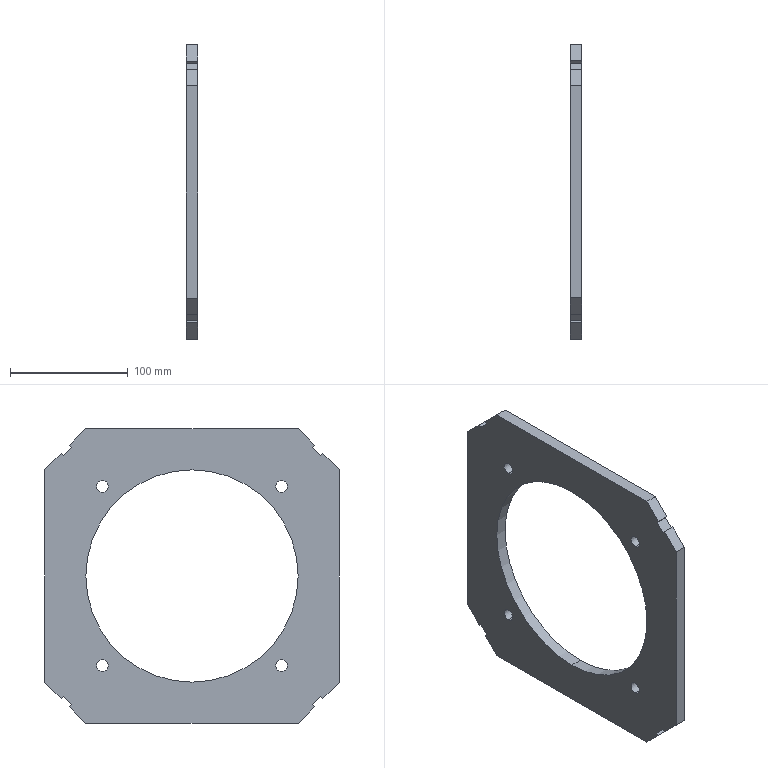Part | STEP file | Produce dryer HY-40-M-701 | 1 solid | 36 faces | box 10 x 250 x 250 mm | volume 341607 mm3 | plane 26 | cylinder 10 | commonest cylinder face diameters 10 x8 180.1 x2
STEP:
#1=CARTESIAN_POINT('',(10.,0.,90.05));
#2=VERTEX_POINT('',#1);
#3=CARTESIAN_POINT('',(10.,0.,-90.05));
#4=VERTEX_POINT('',#3);
#5=CARTESIAN_POINT('',(10.,0.,0.));
#6=DIRECTION('',(1.,0.,0.));
#7=DIRECTION('',(0.,0.,-1.));
#8=AXIS2_PLACEMENT_3D('',#5,#6,#7);
#9=CIRCLE('',#8,90.05);
#10=EDGE_CURVE('',#2,#4,#9,.T.);
#11=ORIENTED_EDGE('',*,*,#10,.T.);
#12=CARTESIAN_POINT('',(0.,0.,-90.05));
#13=VERTEX_POINT('',#12);
#14=CARTESIAN_POINT('',(10.,0.,-90.05));
#15=DIRECTION('',(-1.,0.,0.));
#16=VECTOR('',#15,1000.);
#17=LINE('',#14,#16);
#18=EDGE_CURVE('',#4,#13,#17,.T.);
#19=ORIENTED_EDGE('',*,*,#18,.T.);
#20=CARTESIAN_POINT('',(0.,0.,90.05));
#21=VERTEX_POINT('',#20);
#22=CARTESIAN_POINT('',(0.,0.,0.));
#23=DIRECTION('',(1.,0.,0.));
#24=DIRECTION('',(0.,0.,-1.));
#25=AXIS2_PLACEMENT_3D('',#22,#23,#24);
#26=CIRCLE('',#25,90.05);
#27=EDGE_CURVE('',#21,#13,#26,.T.);
#28=ORIENTED_EDGE('',*,*,#27,.F.);
#29=CARTESIAN_POINT('',(10.,0.,90.05));
#30=DIRECTION('',(-1.,0.,0.));
#31=VECTOR('',#30,1000.);
#32=LINE('',#29,#31);
#33=EDGE_CURVE('',#2,#21,#32,.T.);
#34=ORIENTED_EDGE('',*,*,#33,.F.);
#35=EDGE_LOOP('',(#11,#19,#28,#34));
#36=FACE_OUTER_BOUND('',#35,.T.);
#37=CARTESIAN_POINT('',(10.,0.,0.));
#38=DIRECTION('',(-1.,0.,0.));
#39=DIRECTION('',(0.,0.,1.));
#40=AXIS2_PLACEMENT_3D('',#37,#38,#39);
#41=CYLINDRICAL_SURFACE('',#40,90.05);
#42=ADVANCED_FACE('',(#36),#41,.F.);
#43=CARTESIAN_POINT('',(10.,-76.014,-71.014));
#44=VERTEX_POINT('',#43);
#45=CARTESIAN_POINT('',(10.,-76.014,-81.014));
#46=VERTEX_POINT('',#45);
#47=CARTESIAN_POINT('',(10.,-76.014,-76.014));
#48=DIRECTION('',(1.,0.,0.));
#49=DIRECTION('',(0.,0.,-1.));
#50=AXIS2_PLACEMENT_3D('',#47,#48,#49);
#51=CIRCLE('',#50,5.);
#52=EDGE_CURVE('',#44,#46,#51,.T.);
#53=ORIENTED_EDGE('',*,*,#52,.T.);
#54=CARTESIAN_POINT('',(0.,-76.014,-81.014));
#55=VERTEX_POINT('',#54);
#56=CARTESIAN_POINT('',(10.,-76.014,-81.014));
#57=DIRECTION('',(-1.,0.,0.));
#58=VECTOR('',#57,1000.);
#59=LINE('',#56,#58);
#60=EDGE_CURVE('',#46,#55,#59,.T.);
#61=ORIENTED_EDGE('',*,*,#60,.T.);
#62=CARTESIAN_POINT('',(0.,-76.014,-71.014));
#63=VERTEX_POINT('',#62);
#64=CARTESIAN_POINT('',(0.,-76.014,-76.014));
#65=DIRECTION('',(1.,0.,0.));
#66=DIRECTION('',(0.,0.,-1.));
#67=AXIS2_PLACEMENT_3D('',#64,#65,#66);
#68=CIRCLE('',#67,5.);
#69=EDGE_CURVE('',#63,#55,#68,.T.);
#70=ORIENTED_EDGE('',*,*,#69,.F.);
#71=CARTESIAN_POINT('',(10.,-76.014,-71.014));
#72=DIRECTION('',(-1.,0.,0.));
#73=VECTOR('',#72,1000.);
#74=LINE('',#71,#73);
#75=EDGE_CURVE('',#44,#63,#74,.T.);
#76=ORIENTED_EDGE('',*,*,#75,.F.);
#77=EDGE_LOOP('',(#53,#61,#70,#76));
#78=FACE_OUTER_BOUND('',#77,.T.);
#79=CARTESIAN_POINT('',(10.,-76.014,-76.014));
#80=DIRECTION('',(-1.,0.,0.));
#81=DIRECTION('',(0.,0.,1.));
#82=AXIS2_PLACEMENT_3D('',#79,#80,#81);
#83=CYLINDRICAL_SURFACE('',#82,5.);
#84=ADVANCED_FACE('',(#78),#83,.F.);
#85=CARTESIAN_POINT('',(10.,-76.014,81.014));
#86=VERTEX_POINT('',#85);
#87=CARTESIAN_POINT('',(10.,-76.014,71.014));
#88=VERTEX_POINT('',#87);
#89=CARTESIAN_POINT('',(10.,-76.014,76.014));
#90=DIRECTION('',(1.,0.,0.));
#91=DIRECTION('',(0.,0.,-1.));
#92=AXIS2_PLACEMENT_3D('',#89,#90,#91);
#93=CIRCLE('',#92,5.);
#94=EDGE_CURVE('',#86,#88,#93,.T.);
#95=ORIENTED_EDGE('',*,*,#94,.T.);
#96=CARTESIAN_POINT('',(0.,-76.014,71.014));
#97=VERTEX_POINT('',#96);
#98=CARTESIAN_POINT('',(10.,-76.014,71.014));
#99=DIRECTION('',(-1.,0.,0.));
#100=VECTOR('',#99,1000.);
#101=LINE('',#98,#100);
#102=EDGE_CURVE('',#88,#97,#101,.T.);
#103=ORIENTED_EDGE('',*,*,#102,.T.);
#104=CARTESIAN_POINT('',(0.,-76.014,81.014));
#105=VERTEX_POINT('',#104);
#106=CARTESIAN_POINT('',(0.,-76.014,76.014));
#107=DIRECTION('',(1.,0.,0.));
#108=DIRECTION('',(0.,0.,-1.));
#109=AXIS2_PLACEMENT_3D('',#106,#107,#108);
#110=CIRCLE('',#109,5.);
#111=EDGE_CURVE('',#105,#97,#110,.T.);
#112=ORIENTED_EDGE('',*,*,#111,.F.);
#113=CARTESIAN_POINT('',(10.,-76.014,81.014));
#114=DIRECTION('',(-1.,0.,0.));
#115=VECTOR('',#114,1000.);
#116=LINE('',#113,#115);
#117=EDGE_CURVE('',#86,#105,#116,.T.);
#118=ORIENTED_EDGE('',*,*,#117,.F.);
#119=EDGE_LOOP('',(#95,#103,#112,#118));
#120=FACE_OUTER_BOUND('',#119,.T.);
#121=CARTESIAN_POINT('',(10.,-76.014,76.014));
#122=DIRECTION('',(-1.,0.,0.));
#123=DIRECTION('',(0.,0.,1.));
#124=AXIS2_PLACEMENT_3D('',#121,#122,#123);
#125=CYLINDRICAL_SURFACE('',#124,5.);
#126=ADVANCED_FACE('',(#120),#125,.F.);
#127=CARTESIAN_POINT('',(10.,76.014,-71.014));
#128=VERTEX_POINT('',#127);
#129=CARTESIAN_POINT('',(10.,76.014,-81.014));
#130=VERTEX_POINT('',#129);
#131=CARTESIAN_POINT('',(10.,76.014,-76.014));
#132=DIRECTION('',(1.,0.,0.));
#133=DIRECTION('',(0.,0.,-1.));
#134=AXIS2_PLACEMENT_3D('',#131,#132,#133);
#135=CIRCLE('',#134,5.);
#136=EDGE_CURVE('',#128,#130,#135,.T.);
#137=ORIENTED_EDGE('',*,*,#136,.T.);
#138=CARTESIAN_POINT('',(0.,76.014,-81.014));
#139=VERTEX_POINT('',#138);
#140=CARTESIAN_POINT('',(10.,76.014,-81.014));
#141=DIRECTION('',(-1.,0.,0.));
#142=VECTOR('',#141,1000.);
#143=LINE('',#140,#142);
#144=EDGE_CURVE('',#130,#139,#143,.T.);
#145=ORIENTED_EDGE('',*,*,#144,.T.);
#146=CARTESIAN_POINT('',(0.,76.014,-71.014));
#147=VERTEX_POINT('',#146);
#148=CARTESIAN_POINT('',(0.,76.014,-76.014));
#149=DIRECTION('',(1.,0.,0.));
#150=DIRECTION('',(0.,0.,-1.));
#151=AXIS2_PLACEMENT_3D('',#148,#149,#150);
#152=CIRCLE('',#151,5.);
#153=EDGE_CURVE('',#147,#139,#152,.T.);
#154=ORIENTED_EDGE('',*,*,#153,.F.);
#155=CARTESIAN_POINT('',(10.,76.014,-71.014));
#156=DIRECTION('',(-1.,0.,0.));
#157=VECTOR('',#156,1000.);
#158=LINE('',#155,#157);
#159=EDGE_CURVE('',#128,#147,#158,.T.);
#160=ORIENTED_EDGE('',*,*,#159,.F.);
#161=EDGE_LOOP('',(#137,#145,#154,#160));
#162=FACE_OUTER_BOUND('',#161,.T.);
#163=CARTESIAN_POINT('',(10.,76.014,-76.014));
#164=DIRECTION('',(-1.,0.,0.));
#165=DIRECTION('',(0.,0.,1.));
#166=AXIS2_PLACEMENT_3D('',#163,#164,#165);
#167=CYLINDRICAL_SURFACE('',#166,5.);
#168=ADVANCED_FACE('',(#162),#167,.F.);
#169=CARTESIAN_POINT('',(10.,76.014,81.014));
#170=VERTEX_POINT('',#169);
#171=CARTESIAN_POINT('',(10.,76.014,71.014));
#172=VERTEX_POINT('',#171);
#173=CARTESIAN_POINT('',(10.,76.014,76.014));
#174=DIRECTION('',(1.,0.,0.));
#175=DIRECTION('',(0.,0.,-1.));
#176=AXIS2_PLACEMENT_3D('',#173,#174,#175);
#177=CIRCLE('',#176,5.);
#178=EDGE_CURVE('',#170,#172,#177,.T.);
#179=ORIENTED_EDGE('',*,*,#178,.T.);
#180=CARTESIAN_POINT('',(0.,76.014,71.014));
#181=VERTEX_POINT('',#180);
#182=CARTESIAN_POINT('',(10.,76.014,71.014));
#183=DIRECTION('',(-1.,0.,0.));
#184=VECTOR('',#183,1000.);
#185=LINE('',#182,#184);
#186=EDGE_CURVE('',#172,#181,#185,.T.);
#187=ORIENTED_EDGE('',*,*,#186,.T.);
#188=CARTESIAN_POINT('',(0.,76.014,81.014));
#189=VERTEX_POINT('',#188);
#190=CARTESIAN_POINT('',(0.,76.014,76.014));
#191=DIRECTION('',(1.,0.,0.));
#192=DIRECTION('',(0.,0.,-1.));
#193=AXIS2_PLACEMENT_3D('',#190,#191,#192);
#194=CIRCLE('',#193,5.);
#195=EDGE_CURVE('',#189,#181,#194,.T.);
#196=ORIENTED_EDGE('',*,*,#195,.F.);
#197=CARTESIAN_POINT('',(10.,76.014,81.014));
#198=DIRECTION('',(-1.,0.,0.));
#199=VECTOR('',#198,1000.);
#200=LINE('',#197,#199);
#201=EDGE_CURVE('',#170,#189,#200,.T.);
#202=ORIENTED_EDGE('',*,*,#201,.F.);
#203=EDGE_LOOP('',(#179,#187,#196,#202));
#204=FACE_OUTER_BOUND('',#203,.T.);
#205=CARTESIAN_POINT('',(10.,76.014,76.014));
#206=DIRECTION('',(-1.,0.,0.));
#207=DIRECTION('',(0.,0.,1.));
#208=AXIS2_PLACEMENT_3D('',#205,#206,#207);
#209=CYLINDRICAL_SURFACE('',#208,5.);
#210=ADVANCED_FACE('',(#204),#209,.F.);
#211=ORIENTED_EDGE('',*,*,#52,.F.);
#212=CARTESIAN_POINT('',(10.,-76.014,-76.014));
#213=DIRECTION('',(1.,0.,0.));
#214=DIRECTION('',(0.,0.,-1.));
#215=AXIS2_PLACEMENT_3D('',#212,#213,#214);
#216=CIRCLE('',#215,5.);
#217=EDGE_CURVE('',#46,#44,#216,.T.);
#218=ORIENTED_EDGE('',*,*,#217,.F.);
#219=EDGE_LOOP('',(#211,#218));
#220=FACE_BOUND('',#219,.T.);
#221=ORIENTED_EDGE('',*,*,#136,.F.);
#222=CARTESIAN_POINT('',(10.,76.014,-76.014));
#223=DIRECTION('',(1.,0.,0.));
#224=DIRECTION('',(0.,0.,-1.));
#225=AXIS2_PLACEMENT_3D('',#222,#223,#224);
#226=CIRCLE('',#225,5.);
#227=EDGE_CURVE('',#130,#128,#226,.T.);
#228=ORIENTED_EDGE('',*,*,#227,.F.);
#229=EDGE_LOOP('',(#221,#228));
#230=FACE_BOUND('',#229,.T.);
#231=ORIENTED_EDGE('',*,*,#178,.F.);
#232=CARTESIAN_POINT('',(10.,76.014,76.014));
#233=DIRECTION('',(1.,0.,0.));
#234=DIRECTION('',(0.,0.,-1.));
#235=AXIS2_PLACEMENT_3D('',#232,#233,#234);
#236=CIRCLE('',#235,5.);
#237=EDGE_CURVE('',#172,#170,#236,.T.);
#238=ORIENTED_EDGE('',*,*,#237,.F.);
#239=EDGE_LOOP('',(#231,#238));
#240=FACE_BOUND('',#239,.T.);
#241=ORIENTED_EDGE('',*,*,#94,.F.);
#242=CARTESIAN_POINT('',(10.,-76.014,76.014));
#243=DIRECTION('',(1.,0.,0.));
#244=DIRECTION('',(0.,0.,-1.));
#245=AXIS2_PLACEMENT_3D('',#242,#243,#244);
#246=CIRCLE('',#245,5.);
#247=EDGE_CURVE('',#88,#86,#246,.T.);
#248=ORIENTED_EDGE('',*,*,#247,.F.);
#249=EDGE_LOOP('',(#241,#248));
#250=FACE_BOUND('',#249,.T.);
#251=ORIENTED_EDGE('',*,*,#10,.F.);
#252=CARTESIAN_POINT('',(10.,0.,0.));
#253=DIRECTION('',(1.,0.,0.));
#254=DIRECTION('',(0.,0.,-1.));
#255=AXIS2_PLACEMENT_3D('',#252,#253,#254);
#256=CIRCLE('',#255,90.05);
#257=EDGE_CURVE('',#4,#2,#256,.T.);
#258=ORIENTED_EDGE('',*,*,#257,.F.);
#259=EDGE_LOOP('',(#251,#258));
#260=FACE_BOUND('',#259,.T.);
#261=CARTESIAN_POINT('',(10.,109.268,-102.197));
#262=VERTEX_POINT('',#261);
#263=CARTESIAN_POINT('',(10.,102.197,-109.268));
#264=VERTEX_POINT('',#263);
#265=CARTESIAN_POINT('',(10.,109.268,-102.197));
#266=DIRECTION('',(0.,-0.7071,-0.7071));
#267=VECTOR('',#266,1000.);
#268=LINE('',#265,#267);
#269=EDGE_CURVE('',#262,#264,#268,.T.);
#270=ORIENTED_EDGE('',*,*,#269,.F.);
#271=CARTESIAN_POINT('',(10.,111.036,-103.964));
#272=VERTEX_POINT('',#271);
#273=CARTESIAN_POINT('',(10.,111.036,-103.964));
#274=DIRECTION('',(0.,-0.7071,0.7071));
#275=VECTOR('',#274,1000.);
#276=LINE('',#273,#275);
#277=EDGE_CURVE('',#272,#262,#276,.T.);
#278=ORIENTED_EDGE('',*,*,#277,.F.);
#279=CARTESIAN_POINT('',(10.,125.,-90.));
#280=VERTEX_POINT('',#279);
#281=CARTESIAN_POINT('',(10.,107.5,-107.5));
#282=DIRECTION('',(0.,0.7071,0.7071));
#283=VECTOR('',#282,1000.);
#284=LINE('',#281,#283);
#285=EDGE_CURVE('',#272,#280,#284,.T.);
#286=ORIENTED_EDGE('',*,*,#285,.T.);
#287=CARTESIAN_POINT('',(10.,125.,90.));
#288=VERTEX_POINT('',#287);
#289=CARTESIAN_POINT('',(10.,125.,125.));
#290=DIRECTION('',(0.,0.,1.));
#291=VECTOR('',#290,1000.);
#292=LINE('',#289,#291);
#293=EDGE_CURVE('',#280,#288,#292,.T.);
#294=ORIENTED_EDGE('',*,*,#293,.T.);
#295=CARTESIAN_POINT('',(10.,111.036,103.964));
#296=VERTEX_POINT('',#295);
#297=CARTESIAN_POINT('',(10.,-17.5,232.5));
#298=DIRECTION('',(0.,-0.7071,0.7071));
#299=VECTOR('',#298,1000.);
#300=LINE('',#297,#299);
#301=EDGE_CURVE('',#288,#296,#300,.T.);
#302=ORIENTED_EDGE('',*,*,#301,.T.);
#303=CARTESIAN_POINT('',(10.,109.268,102.197));
#304=VERTEX_POINT('',#303);
#305=CARTESIAN_POINT('',(10.,111.036,103.964));
#306=DIRECTION('',(0.,0.7071,0.7071));
#307=VECTOR('',#306,1000.);
#308=LINE('',#305,#307);
#309=EDGE_CURVE('',#304,#296,#308,.T.);
#310=ORIENTED_EDGE('',*,*,#309,.F.);
#311=CARTESIAN_POINT('',(10.,102.197,109.268));
#312=VERTEX_POINT('',#311);
#313=CARTESIAN_POINT('',(10.,109.268,102.197));
#314=DIRECTION('',(0.,0.7071,-0.7071));
#315=VECTOR('',#314,1000.);
#316=LINE('',#313,#315);
#317=EDGE_CURVE('',#312,#304,#316,.T.);
#318=ORIENTED_EDGE('',*,*,#317,.F.);
#319=CARTESIAN_POINT('',(10.,103.964,111.036));
#320=VERTEX_POINT('',#319);
#321=CARTESIAN_POINT('',(10.,102.197,109.268));
#322=DIRECTION('',(0.,-0.7071,-0.7071));
#323=VECTOR('',#322,1000.);
#324=LINE('',#321,#323);
#325=EDGE_CURVE('',#320,#312,#324,.T.);
#326=ORIENTED_EDGE('',*,*,#325,.F.);
#327=CARTESIAN_POINT('',(10.,90.,125.));
#328=VERTEX_POINT('',#327);
#329=CARTESIAN_POINT('',(10.,-17.5,232.5));
#330=DIRECTION('',(0.,-0.7071,0.7071));
#331=VECTOR('',#330,1000.);
#332=LINE('',#329,#331);
#333=EDGE_CURVE('',#320,#328,#332,.T.);
#334=ORIENTED_EDGE('',*,*,#333,.T.);
#335=CARTESIAN_POINT('',(10.,-90.,125.));
#336=VERTEX_POINT('',#335);
#337=CARTESIAN_POINT('',(10.,125.,125.));
#338=DIRECTION('',(0.,-1.,0.));
#339=VECTOR('',#338,1000.);
#340=LINE('',#337,#339);
#341=EDGE_CURVE('',#328,#336,#340,.T.);
#342=ORIENTED_EDGE('',*,*,#341,.T.);
#343=CARTESIAN_POINT('',(10.,-103.964,111.036));
#344=VERTEX_POINT('',#343);
#345=CARTESIAN_POINT('',(10.,-107.5,107.5));
#346=DIRECTION('',(0.,-0.7071,-0.7071));
#347=VECTOR('',#346,1000.);
#348=LINE('',#345,#347);
#349=EDGE_CURVE('',#336,#344,#348,.T.);
#350=ORIENTED_EDGE('',*,*,#349,.T.);
#351=CARTESIAN_POINT('',(10.,-102.197,109.268));
#352=VERTEX_POINT('',#351);
#353=CARTESIAN_POINT('',(10.,-102.197,109.268));
#354=DIRECTION('',(0.,-0.7071,0.7071));
#355=VECTOR('',#354,1000.);
#356=LINE('',#353,#355);
#357=EDGE_CURVE('',#352,#344,#356,.T.);
#358=ORIENTED_EDGE('',*,*,#357,.F.);
#359=CARTESIAN_POINT('',(10.,-109.268,102.197));
#360=VERTEX_POINT('',#359);
#361=CARTESIAN_POINT('',(10.,-109.268,102.197));
#362=DIRECTION('',(0.,0.7071,0.7071));
#363=VECTOR('',#362,1000.);
#364=LINE('',#361,#363);
#365=EDGE_CURVE('',#360,#352,#364,.T.);
#366=ORIENTED_EDGE('',*,*,#365,.F.);
#367=CARTESIAN_POINT('',(10.,-111.036,103.964));
#368=VERTEX_POINT('',#367);
#369=CARTESIAN_POINT('',(10.,-111.036,103.964));
#370=DIRECTION('',(0.,0.7071,-0.7071));
#371=VECTOR('',#370,1000.);
#372=LINE('',#369,#371);
#373=EDGE_CURVE('',#368,#360,#372,.T.);
#374=ORIENTED_EDGE('',*,*,#373,.F.);
#375=CARTESIAN_POINT('',(10.,-125.,90.));
#376=VERTEX_POINT('',#375);
#377=CARTESIAN_POINT('',(10.,-107.5,107.5));
#378=DIRECTION('',(0.,-0.7071,-0.7071));
#379=VECTOR('',#378,1000.);
#380=LINE('',#377,#379);
#381=EDGE_CURVE('',#368,#376,#380,.T.);
#382=ORIENTED_EDGE('',*,*,#381,.T.);
#383=CARTESIAN_POINT('',(10.,-125.,-90.));
#384=VERTEX_POINT('',#383);
#385=CARTESIAN_POINT('',(10.,-125.,125.));
#386=DIRECTION('',(0.,0.,-1.));
#387=VECTOR('',#386,1000.);
#388=LINE('',#385,#387);
#389=EDGE_CURVE('',#376,#384,#388,.T.);
#390=ORIENTED_EDGE('',*,*,#389,.T.);
#391=CARTESIAN_POINT('',(10.,-111.036,-103.964));
#392=VERTEX_POINT('',#391);
#393=CARTESIAN_POINT('',(10.,-232.5,17.5));
#394=DIRECTION('',(0.,0.7071,-0.7071));
#395=VECTOR('',#394,1000.);
#396=LINE('',#393,#395);
#397=EDGE_CURVE('',#384,#392,#396,.T.);
#398=ORIENTED_EDGE('',*,*,#397,.T.);
#399=CARTESIAN_POINT('',(10.,-109.268,-102.197));
#400=VERTEX_POINT('',#399);
#401=CARTESIAN_POINT('',(10.,-111.036,-103.964));
#402=DIRECTION('',(0.,-0.7071,-0.7071));
#403=VECTOR('',#402,1000.);
#404=LINE('',#401,#403);
#405=EDGE_CURVE('',#400,#392,#404,.T.);
#406=ORIENTED_EDGE('',*,*,#405,.F.);
#407=CARTESIAN_POINT('',(10.,-102.197,-109.268));
#408=VERTEX_POINT('',#407);
#409=CARTESIAN_POINT('',(10.,-109.268,-102.197));
#410=DIRECTION('',(0.,-0.7071,0.7071));
#411=VECTOR('',#410,1000.);
#412=LINE('',#409,#411);
#413=EDGE_CURVE('',#408,#400,#412,.T.);
#414=ORIENTED_EDGE('',*,*,#413,.F.);
#415=CARTESIAN_POINT('',(10.,-103.964,-111.036));
#416=VERTEX_POINT('',#415);
#417=CARTESIAN_POINT('',(10.,-102.197,-109.268));
#418=DIRECTION('',(0.,0.7071,0.7071));
#419=VECTOR('',#418,1000.);
#420=LINE('',#417,#419);
#421=EDGE_CURVE('',#416,#408,#420,.T.);
#422=ORIENTED_EDGE('',*,*,#421,.F.);
#423=CARTESIAN_POINT('',(10.,-90.,-125.));
#424=VERTEX_POINT('',#423);
#425=CARTESIAN_POINT('',(10.,-232.5,17.5));
#426=DIRECTION('',(0.,0.7071,-0.7071));
#427=VECTOR('',#426,1000.);
#428=LINE('',#425,#427);
#429=EDGE_CURVE('',#416,#424,#428,.T.);
#430=ORIENTED_EDGE('',*,*,#429,.T.);
#431=CARTESIAN_POINT('',(10.,90.,-125.));
#432=VERTEX_POINT('',#431);
#433=CARTESIAN_POINT('',(10.,125.,-125.));
#434=DIRECTION('',(0.,1.,0.));
#435=VECTOR('',#434,1000.);
#436=LINE('',#433,#435);
#437=EDGE_CURVE('',#424,#432,#436,.T.);
#438=ORIENTED_EDGE('',*,*,#437,.T.);
#439=CARTESIAN_POINT('',(10.,103.964,-111.036));
#440=VERTEX_POINT('',#439);
#441=CARTESIAN_POINT('',(10.,107.5,-107.5));
#442=DIRECTION('',(0.,0.7071,0.7071));
#443=VECTOR('',#442,1000.);
#444=LINE('',#441,#443);
#445=EDGE_CURVE('',#432,#440,#444,.T.);
#446=ORIENTED_EDGE('',*,*,#445,.T.);
#447=CARTESIAN_POINT('',(10.,102.197,-109.268));
#448=DIRECTION('',(0.,0.7071,-0.7071));
#449=VECTOR('',#448,1000.);
#450=LINE('',#447,#449);
#451=EDGE_CURVE('',#264,#440,#450,.T.);
#452=ORIENTED_EDGE('',*,*,#451,.F.);
#453=EDGE_LOOP('',(#270,#278,#286,#294,#302,#310,#318,#326,#334,#342,#350,#358,#366,#374,#382,#390,#398,#406,#414,#422,#430,#438,#446,#452));
#454=FACE_OUTER_BOUND('',#453,.T.);
#455=CARTESIAN_POINT('',(10.,-125.,125.));
#456=DIRECTION('',(1.,0.,0.));
#457=DIRECTION('',(0.,0.,-1.));
#458=AXIS2_PLACEMENT_3D('',#455,#456,#457);
#459=PLANE('',#458);
#460=ADVANCED_FACE('',(#220,#230,#240,#250,#260,#454),#459,.T.);
#461=ORIENTED_EDGE('',*,*,#195,.T.);
#462=CARTESIAN_POINT('',(0.,76.014,76.014));
#463=DIRECTION('',(1.,0.,0.));
#464=DIRECTION('',(0.,0.,-1.));
#465=AXIS2_PLACEMENT_3D('',#462,#463,#464);
#466=CIRCLE('',#465,5.);
#467=EDGE_CURVE('',#181,#189,#466,.T.);
#468=ORIENTED_EDGE('',*,*,#467,.T.);
#469=EDGE_LOOP('',(#461,#468));
#470=FACE_BOUND('',#469,.T.);
#471=ORIENTED_EDGE('',*,*,#153,.T.);
#472=CARTESIAN_POINT('',(0.,76.014,-76.014));
#473=DIRECTION('',(1.,0.,0.));
#474=DIRECTION('',(0.,0.,-1.));
#475=AXIS2_PLACEMENT_3D('',#472,#473,#474);
#476=CIRCLE('',#475,5.);
#477=EDGE_CURVE('',#139,#147,#476,.T.);
#478=ORIENTED_EDGE('',*,*,#477,.T.);
#479=EDGE_LOOP('',(#471,#478));
#480=FACE_BOUND('',#479,.T.);
#481=ORIENTED_EDGE('',*,*,#111,.T.);
#482=CARTESIAN_POINT('',(0.,-76.014,76.014));
#483=DIRECTION('',(1.,0.,0.));
#484=DIRECTION('',(0.,0.,-1.));
#485=AXIS2_PLACEMENT_3D('',#482,#483,#484);
#486=CIRCLE('',#485,5.);
#487=EDGE_CURVE('',#97,#105,#486,.T.);
#488=ORIENTED_EDGE('',*,*,#487,.T.);
#489=EDGE_LOOP('',(#481,#488));
#490=FACE_BOUND('',#489,.T.);
#491=ORIENTED_EDGE('',*,*,#69,.T.);
#492=CARTESIAN_POINT('',(0.,-76.014,-76.014));
#493=DIRECTION('',(1.,0.,0.));
#494=DIRECTION('',(0.,0.,-1.));
#495=AXIS2_PLACEMENT_3D('',#492,#493,#494);
#496=CIRCLE('',#495,5.);
#497=EDGE_CURVE('',#55,#63,#496,.T.);
#498=ORIENTED_EDGE('',*,*,#497,.T.);
#499=EDGE_LOOP('',(#491,#498));
#500=FACE_BOUND('',#499,.T.);
#501=ORIENTED_EDGE('',*,*,#27,.T.);
#502=CARTESIAN_POINT('',(0.,0.,0.));
#503=DIRECTION('',(1.,0.,0.));
#504=DIRECTION('',(0.,0.,-1.));
#505=AXIS2_PLACEMENT_3D('',#502,#503,#504);
#506=CIRCLE('',#505,90.05);
#507=EDGE_CURVE('',#13,#21,#506,.T.);
#508=ORIENTED_EDGE('',*,*,#507,.T.);
#509=EDGE_LOOP('',(#501,#508));
#510=FACE_BOUND('',#509,.T.);
#511=CARTESIAN_POINT('',(0.,111.036,-103.964));
#512=VERTEX_POINT('',#511);
#513=CARTESIAN_POINT('',(0.,109.268,-102.197));
#514=VERTEX_POINT('',#513);
#515=CARTESIAN_POINT('',(0.,111.036,-103.964));
#516=DIRECTION('',(0.,-0.7071,0.7071));
#517=VECTOR('',#516,1000.);
#518=LINE('',#515,#517);
#519=EDGE_CURVE('',#512,#514,#518,.T.);
#520=ORIENTED_EDGE('',*,*,#519,.T.);
#521=CARTESIAN_POINT('',(0.,102.197,-109.268));
#522=VERTEX_POINT('',#521);
#523=CARTESIAN_POINT('',(0.,109.268,-102.197));
#524=DIRECTION('',(0.,-0.7071,-0.7071));
#525=VECTOR('',#524,1000.);
#526=LINE('',#523,#525);
#527=EDGE_CURVE('',#514,#522,#526,.T.);
#528=ORIENTED_EDGE('',*,*,#527,.T.);
#529=CARTESIAN_POINT('',(0.,103.964,-111.036));
#530=VERTEX_POINT('',#529);
#531=CARTESIAN_POINT('',(0.,102.197,-109.268));
#532=DIRECTION('',(0.,0.7071,-0.7071));
#533=VECTOR('',#532,1000.);
#534=LINE('',#531,#533);
#535=EDGE_CURVE('',#522,#530,#534,.T.);
#536=ORIENTED_EDGE('',*,*,#535,.T.);
#537=CARTESIAN_POINT('',(0.,90.,-125.));
#538=VERTEX_POINT('',#537);
#539=CARTESIAN_POINT('',(0.,125.,-90.));
#540=DIRECTION('',(0.,-0.7071,-0.7071));
#541=VECTOR('',#540,1000.);
#542=LINE('',#539,#541);
#543=EDGE_CURVE('',#530,#538,#542,.T.);
#544=ORIENTED_EDGE('',*,*,#543,.T.);
#545=CARTESIAN_POINT('',(0.,-90.,-125.));
#546=VERTEX_POINT('',#545);
#547=CARTESIAN_POINT('',(0.,125.,-125.));
#548=DIRECTION('',(0.,1.,0.));
#549=VECTOR('',#548,1000.);
#550=LINE('',#547,#549);
#551=EDGE_CURVE('',#546,#538,#550,.T.);
#552=ORIENTED_EDGE('',*,*,#551,.F.);
#553=CARTESIAN_POINT('',(0.,-103.964,-111.036));
#554=VERTEX_POINT('',#553);
#555=CARTESIAN_POINT('',(0.,-90.,-125.));
#556=DIRECTION('',(0.,-0.7071,0.7071));
#557=VECTOR('',#556,1000.);
#558=LINE('',#555,#557);
#559=EDGE_CURVE('',#546,#554,#558,.T.);
#560=ORIENTED_EDGE('',*,*,#559,.T.);
#561=CARTESIAN_POINT('',(0.,-102.197,-109.268));
#562=VERTEX_POINT('',#561);
#563=CARTESIAN_POINT('',(0.,-102.197,-109.268));
#564=DIRECTION('',(0.,0.7071,0.7071));
#565=VECTOR('',#564,1000.);
#566=LINE('',#563,#565);
#567=EDGE_CURVE('',#554,#562,#566,.T.);
#568=ORIENTED_EDGE('',*,*,#567,.T.);
#569=CARTESIAN_POINT('',(0.,-109.268,-102.197));
#570=VERTEX_POINT('',#569);
#571=CARTESIAN_POINT('',(0.,-109.268,-102.197));
#572=DIRECTION('',(0.,-0.7071,0.7071));
#573=VECTOR('',#572,1000.);
#574=LINE('',#571,#573);
#575=EDGE_CURVE('',#562,#570,#574,.T.);
#576=ORIENTED_EDGE('',*,*,#575,.T.);
#577=CARTESIAN_POINT('',(0.,-111.036,-103.964));
#578=VERTEX_POINT('',#577);
#579=CARTESIAN_POINT('',(0.,-111.036,-103.964));
#580=DIRECTION('',(0.,-0.7071,-0.7071));
#581=VECTOR('',#580,1000.);
#582=LINE('',#579,#581);
#583=EDGE_CURVE('',#570,#578,#582,.T.);
#584=ORIENTED_EDGE('',*,*,#583,.T.);
#585=CARTESIAN_POINT('',(0.,-125.,-90.));
#586=VERTEX_POINT('',#585);
#587=CARTESIAN_POINT('',(0.,-90.,-125.));
#588=DIRECTION('',(0.,-0.7071,0.7071));
#589=VECTOR('',#588,1000.);
#590=LINE('',#587,#589);
#591=EDGE_CURVE('',#578,#586,#590,.T.);
#592=ORIENTED_EDGE('',*,*,#591,.T.);
#593=CARTESIAN_POINT('',(0.,-125.,90.));
#594=VERTEX_POINT('',#593);
#595=CARTESIAN_POINT('',(0.,-125.,125.));
#596=DIRECTION('',(0.,0.,-1.));
#597=VECTOR('',#596,1000.);
#598=LINE('',#595,#597);
#599=EDGE_CURVE('',#594,#586,#598,.T.);
#600=ORIENTED_EDGE('',*,*,#599,.F.);
#601=CARTESIAN_POINT('',(0.,-111.036,103.964));
#602=VERTEX_POINT('',#601);
#603=CARTESIAN_POINT('',(0.,-125.,90.));
#604=DIRECTION('',(0.,0.7071,0.7071));
#605=VECTOR('',#604,1000.);
#606=LINE('',#603,#605);
#607=EDGE_CURVE('',#594,#602,#606,.T.);
#608=ORIENTED_EDGE('',*,*,#607,.T.);
#609=CARTESIAN_POINT('',(0.,-109.268,102.197));
#610=VERTEX_POINT('',#609);
#611=CARTESIAN_POINT('',(0.,-111.036,103.964));
#612=DIRECTION('',(0.,0.7071,-0.7071));
#613=VECTOR('',#612,1000.);
#614=LINE('',#611,#613);
#615=EDGE_CURVE('',#602,#610,#614,.T.);
#616=ORIENTED_EDGE('',*,*,#615,.T.);
#617=CARTESIAN_POINT('',(0.,-102.197,109.268));
#618=VERTEX_POINT('',#617);
#619=CARTESIAN_POINT('',(0.,-109.268,102.197));
#620=DIRECTION('',(0.,0.7071,0.7071));
#621=VECTOR('',#620,1000.);
#622=LINE('',#619,#621);
#623=EDGE_CURVE('',#610,#618,#622,.T.);
#624=ORIENTED_EDGE('',*,*,#623,.T.);
#625=CARTESIAN_POINT('',(0.,-103.964,111.036));
#626=VERTEX_POINT('',#625);
#627=CARTESIAN_POINT('',(0.,-102.197,109.268));
#628=DIRECTION('',(0.,-0.7071,0.7071));
#629=VECTOR('',#628,1000.);
#630=LINE('',#627,#629);
#631=EDGE_CURVE('',#618,#626,#630,.T.);
#632=ORIENTED_EDGE('',*,*,#631,.T.);
#633=CARTESIAN_POINT('',(0.,-90.,125.));
#634=VERTEX_POINT('',#633);
#635=CARTESIAN_POINT('',(0.,-125.,90.));
#636=DIRECTION('',(0.,0.7071,0.7071));
#637=VECTOR('',#636,1000.);
#638=LINE('',#635,#637);
#639=EDGE_CURVE('',#626,#634,#638,.T.);
#640=ORIENTED_EDGE('',*,*,#639,.T.);
#641=CARTESIAN_POINT('',(0.,90.,125.));
#642=VERTEX_POINT('',#641);
#643=CARTESIAN_POINT('',(0.,125.,125.));
#644=DIRECTION('',(0.,-1.,0.));
#645=VECTOR('',#644,1000.);
#646=LINE('',#643,#645);
#647=EDGE_CURVE('',#642,#634,#646,.T.);
#648=ORIENTED_EDGE('',*,*,#647,.F.);
#649=CARTESIAN_POINT('',(0.,103.964,111.036));
#650=VERTEX_POINT('',#649);
#651=CARTESIAN_POINT('',(0.,90.,125.));
#652=DIRECTION('',(0.,0.7071,-0.7071));
#653=VECTOR('',#652,1000.);
#654=LINE('',#651,#653);
#655=EDGE_CURVE('',#642,#650,#654,.T.);
#656=ORIENTED_EDGE('',*,*,#655,.T.);
#657=CARTESIAN_POINT('',(0.,102.197,109.268));
#658=VERTEX_POINT('',#657);
#659=CARTESIAN_POINT('',(0.,102.197,109.268));
#660=DIRECTION('',(0.,-0.7071,-0.7071));
#661=VECTOR('',#660,1000.);
#662=LINE('',#659,#661);
#663=EDGE_CURVE('',#650,#658,#662,.T.);
#664=ORIENTED_EDGE('',*,*,#663,.T.);
#665=CARTESIAN_POINT('',(0.,109.268,102.197));
#666=VERTEX_POINT('',#665);
#667=CARTESIAN_POINT('',(0.,109.268,102.197));
#668=DIRECTION('',(0.,0.7071,-0.7071));
#669=VECTOR('',#668,1000.);
#670=LINE('',#667,#669);
#671=EDGE_CURVE('',#658,#666,#670,.T.);
#672=ORIENTED_EDGE('',*,*,#671,.T.);
#673=CARTESIAN_POINT('',(0.,111.036,103.964));
#674=VERTEX_POINT('',#673);
#675=CARTESIAN_POINT('',(0.,111.036,103.964));
#676=DIRECTION('',(0.,0.7071,0.7071));
#677=VECTOR('',#676,1000.);
#678=LINE('',#675,#677);
#679=EDGE_CURVE('',#666,#674,#678,.T.);
#680=ORIENTED_EDGE('',*,*,#679,.T.);
#681=CARTESIAN_POINT('',(0.,125.,90.));
#682=VERTEX_POINT('',#681);
#683=CARTESIAN_POINT('',(0.,90.,125.));
#684=DIRECTION('',(0.,0.7071,-0.7071));
#685=VECTOR('',#684,1000.);
#686=LINE('',#683,#685);
#687=EDGE_CURVE('',#674,#682,#686,.T.);
#688=ORIENTED_EDGE('',*,*,#687,.T.);
#689=CARTESIAN_POINT('',(0.,125.,-90.));
#690=VERTEX_POINT('',#689);
#691=CARTESIAN_POINT('',(0.,125.,125.));
#692=DIRECTION('',(0.,0.,1.));
#693=VECTOR('',#692,1000.);
#694=LINE('',#691,#693);
#695=EDGE_CURVE('',#690,#682,#694,.T.);
#696=ORIENTED_EDGE('',*,*,#695,.F.);
#697=CARTESIAN_POINT('',(0.,125.,-90.));
#698=DIRECTION('',(0.,-0.7071,-0.7071));
#699=VECTOR('',#698,1000.);
#700=LINE('',#697,#699);
#701=EDGE_CURVE('',#690,#512,#700,.T.);
#702=ORIENTED_EDGE('',*,*,#701,.T.);
#703=EDGE_LOOP('',(#520,#528,#536,#544,#552,#560,#568,#576,#584,#592,#600,#608,#616,#624,#632,#640,#648,#656,#664,#672,#680,#688,#696,#702));
#704=FACE_OUTER_BOUND('',#703,.T.);
#705=CARTESIAN_POINT('',(0.,-125.,125.));
#706=DIRECTION('',(1.,0.,0.));
#707=DIRECTION('',(0.,0.,-1.));
#708=AXIS2_PLACEMENT_3D('',#705,#706,#707);
#709=PLANE('',#708);
#710=ADVANCED_FACE('',(#470,#480,#490,#500,#510,#704),#709,.F.);
#711=ORIENTED_EDGE('',*,*,#285,.F.);
#712=CARTESIAN_POINT('',(10.,111.036,-103.964));
#713=DIRECTION('',(-1.,0.,0.));
#714=VECTOR('',#713,1000.);
#715=LINE('',#712,#714);
#716=EDGE_CURVE('',#272,#512,#715,.T.);
#717=ORIENTED_EDGE('',*,*,#716,.T.);
#718=ORIENTED_EDGE('',*,*,#701,.F.);
#719=CARTESIAN_POINT('',(10.,125.,-90.));
#720=DIRECTION('',(-1.,0.,0.));
#721=VECTOR('',#720,1000.);
#722=LINE('',#719,#721);
#723=EDGE_CURVE('',#280,#690,#722,.T.);
#724=ORIENTED_EDGE('',*,*,#723,.F.);
#725=EDGE_LOOP('',(#711,#717,#718,#724));
#726=FACE_OUTER_BOUND('',#725,.T.);
#727=CARTESIAN_POINT('',(10.,125.,-90.));
#728=DIRECTION('',(0.,-0.7071,0.7071));
#729=DIRECTION('',(-1.,0.,0.));
#730=AXIS2_PLACEMENT_3D('',#727,#728,#729);
#731=PLANE('',#730);
#732=ADVANCED_FACE('',(#726),#731,.F.);
#733=ORIENTED_EDGE('',*,*,#543,.F.);
#734=CARTESIAN_POINT('',(10.,103.964,-111.036));
#735=DIRECTION('',(-1.,0.,0.));
#736=VECTOR('',#735,1000.);
#737=LINE('',#734,#736);
#738=EDGE_CURVE('',#440,#530,#737,.T.);
#739=ORIENTED_EDGE('',*,*,#738,.F.);
#740=ORIENTED_EDGE('',*,*,#445,.F.);
#741=CARTESIAN_POINT('',(10.,90.,-125.));
#742=DIRECTION('',(1.,0.,0.));
#743=VECTOR('',#742,1000.);
#744=LINE('',#741,#743);
#745=EDGE_CURVE('',#538,#432,#744,.T.);
#746=ORIENTED_EDGE('',*,*,#745,.F.);
#747=EDGE_LOOP('',(#733,#739,#740,#746));
#748=FACE_OUTER_BOUND('',#747,.T.);
#749=CARTESIAN_POINT('',(10.,125.,-90.));
#750=DIRECTION('',(0.,-0.7071,0.7071));
#751=DIRECTION('',(-1.,0.,0.));
#752=AXIS2_PLACEMENT_3D('',#749,#750,#751);
#753=PLANE('',#752);
#754=ADVANCED_FACE('',(#748),#753,.F.);
#755=ORIENTED_EDGE('',*,*,#429,.F.);
#756=CARTESIAN_POINT('',(10.,-103.964,-111.036));
#757=DIRECTION('',(-1.,0.,0.));
#758=VECTOR('',#757,1000.);
#759=LINE('',#756,#758);
#760=EDGE_CURVE('',#416,#554,#759,.T.);
#761=ORIENTED_EDGE('',*,*,#760,.T.);
#762=ORIENTED_EDGE('',*,*,#559,.F.);
#763=CARTESIAN_POINT('',(10.,-90.,-125.));
#764=DIRECTION('',(-1.,0.,0.));
#765=VECTOR('',#764,1000.);
#766=LINE('',#763,#765);
#767=EDGE_CURVE('',#424,#546,#766,.T.);
#768=ORIENTED_EDGE('',*,*,#767,.F.);
#769=EDGE_LOOP('',(#755,#761,#762,#768));
#770=FACE_OUTER_BOUND('',#769,.T.);
#771=CARTESIAN_POINT('',(10.,-90.,-125.));
#772=DIRECTION('',(0.,0.7071,0.7071));
#773=DIRECTION('',(-1.,0.,0.));
#774=AXIS2_PLACEMENT_3D('',#771,#772,#773);
#775=PLANE('',#774);
#776=ADVANCED_FACE('',(#770),#775,.F.);
#777=ORIENTED_EDGE('',*,*,#591,.F.);
#778=CARTESIAN_POINT('',(10.,-111.036,-103.964));
#779=DIRECTION('',(-1.,0.,0.));
#780=VECTOR('',#779,1000.);
#781=LINE('',#778,#780);
#782=EDGE_CURVE('',#392,#578,#781,.T.);
#783=ORIENTED_EDGE('',*,*,#782,.F.);
#784=ORIENTED_EDGE('',*,*,#397,.F.);
#785=CARTESIAN_POINT('',(10.,-125.,-90.));
#786=DIRECTION('',(1.,0.,0.));
#787=VECTOR('',#786,1000.);
#788=LINE('',#785,#787);
#789=EDGE_CURVE('',#586,#384,#788,.T.);
#790=ORIENTED_EDGE('',*,*,#789,.F.);
#791=EDGE_LOOP('',(#777,#783,#784,#790));
#792=FACE_OUTER_BOUND('',#791,.T.);
#793=CARTESIAN_POINT('',(10.,-90.,-125.));
#794=DIRECTION('',(0.,0.7071,0.7071));
#795=DIRECTION('',(-1.,0.,0.));
#796=AXIS2_PLACEMENT_3D('',#793,#794,#795);
#797=PLANE('',#796);
#798=ADVANCED_FACE('',(#792),#797,.F.);
#799=ORIENTED_EDGE('',*,*,#381,.F.);
#800=CARTESIAN_POINT('',(10.,-111.036,103.964));
#801=DIRECTION('',(-1.,0.,0.));
#802=VECTOR('',#801,1000.);
#803=LINE('',#800,#802);
#804=EDGE_CURVE('',#368,#602,#803,.T.);
#805=ORIENTED_EDGE('',*,*,#804,.T.);
#806=ORIENTED_EDGE('',*,*,#607,.F.);
#807=CARTESIAN_POINT('',(10.,-125.,90.));
#808=DIRECTION('',(-1.,0.,0.));
#809=VECTOR('',#808,1000.);
#810=LINE('',#807,#809);
#811=EDGE_CURVE('',#376,#594,#810,.T.);
#812=ORIENTED_EDGE('',*,*,#811,.F.);
#813=EDGE_LOOP('',(#799,#805,#806,#812));
#814=FACE_OUTER_BOUND('',#813,.T.);
#815=CARTESIAN_POINT('',(10.,-125.,90.));
#816=DIRECTION('',(0.,0.7071,-0.7071));
#817=DIRECTION('',(-1.,0.,0.));
#818=AXIS2_PLACEMENT_3D('',#815,#816,#817);
#819=PLANE('',#818);
#820=ADVANCED_FACE('',(#814),#819,.F.);
#821=ORIENTED_EDGE('',*,*,#639,.F.);
#822=CARTESIAN_POINT('',(10.,-103.964,111.036));
#823=DIRECTION('',(-1.,0.,0.));
#824=VECTOR('',#823,1000.);
#825=LINE('',#822,#824);
#826=EDGE_CURVE('',#344,#626,#825,.T.);
#827=ORIENTED_EDGE('',*,*,#826,.F.);
#828=ORIENTED_EDGE('',*,*,#349,.F.);
#829=CARTESIAN_POINT('',(10.,-90.,125.));
#830=DIRECTION('',(1.,0.,0.));
#831=VECTOR('',#830,1000.);
#832=LINE('',#829,#831);
#833=EDGE_CURVE('',#634,#336,#832,.T.);
#834=ORIENTED_EDGE('',*,*,#833,.F.);
#835=EDGE_LOOP('',(#821,#827,#828,#834));
#836=FACE_OUTER_BOUND('',#835,.T.);
#837=CARTESIAN_POINT('',(10.,-125.,90.));
#838=DIRECTION('',(0.,0.7071,-0.7071));
#839=DIRECTION('',(-1.,0.,0.));
#840=AXIS2_PLACEMENT_3D('',#837,#838,#839);
#841=PLANE('',#840);
#842=ADVANCED_FACE('',(#836),#841,.F.);
#843=ORIENTED_EDGE('',*,*,#333,.F.);
#844=CARTESIAN_POINT('',(10.,103.964,111.036));
#845=DIRECTION('',(-1.,0.,0.));
#846=VECTOR('',#845,1000.);
#847=LINE('',#844,#846);
#848=EDGE_CURVE('',#320,#650,#847,.T.);
#849=ORIENTED_EDGE('',*,*,#848,.T.);
#850=ORIENTED_EDGE('',*,*,#655,.F.);
#851=CARTESIAN_POINT('',(10.,90.,125.));
#852=DIRECTION('',(-1.,0.,0.));
#853=VECTOR('',#852,1000.);
#854=LINE('',#851,#853);
#855=EDGE_CURVE('',#328,#642,#854,.T.);
#856=ORIENTED_EDGE('',*,*,#855,.F.);
#857=EDGE_LOOP('',(#843,#849,#850,#856));
#858=FACE_OUTER_BOUND('',#857,.T.);
#859=CARTESIAN_POINT('',(10.,90.,125.));
#860=DIRECTION('',(0.,-0.7071,-0.7071));
#861=DIRECTION('',(-1.,0.,0.));
#862=AXIS2_PLACEMENT_3D('',#859,#860,#861);
#863=PLANE('',#862);
#864=ADVANCED_FACE('',(#858),#863,.F.);
#865=ORIENTED_EDGE('',*,*,#687,.F.);
#866=CARTESIAN_POINT('',(10.,111.036,103.964));
#867=DIRECTION('',(-1.,0.,0.));
#868=VECTOR('',#867,1000.);
#869=LINE('',#866,#868);
#870=EDGE_CURVE('',#296,#674,#869,.T.);
#871=ORIENTED_EDGE('',*,*,#870,.F.);
#872=ORIENTED_EDGE('',*,*,#301,.F.);
#873=CARTESIAN_POINT('',(10.,125.,90.));
#874=DIRECTION('',(1.,0.,0.));
#875=VECTOR('',#874,1000.);
#876=LINE('',#873,#875);
#877=EDGE_CURVE('',#682,#288,#876,.T.);
#878=ORIENTED_EDGE('',*,*,#877,.F.);
#879=EDGE_LOOP('',(#865,#871,#872,#878));
#880=FACE_OUTER_BOUND('',#879,.T.);
#881=CARTESIAN_POINT('',(10.,90.,125.));
#882=DIRECTION('',(0.,-0.7071,-0.7071));
#883=DIRECTION('',(-1.,0.,0.));
#884=AXIS2_PLACEMENT_3D('',#881,#882,#883);
#885=PLANE('',#884);
#886=ADVANCED_FACE('',(#880),#885,.F.);
#887=ORIENTED_EDGE('',*,*,#647,.T.);
#888=ORIENTED_EDGE('',*,*,#833,.T.);
#889=ORIENTED_EDGE('',*,*,#341,.F.);
#890=ORIENTED_EDGE('',*,*,#855,.T.);
#891=EDGE_LOOP('',(#887,#888,#889,#890));
#892=FACE_OUTER_BOUND('',#891,.T.);
#893=CARTESIAN_POINT('',(10.,125.,125.));
#894=DIRECTION('',(0.,0.,-1.));
#895=DIRECTION('',(0.,1.,0.));
#896=AXIS2_PLACEMENT_3D('',#893,#894,#895);
#897=PLANE('',#896);
#898=ADVANCED_FACE('',(#892),#897,.F.);
#899=ORIENTED_EDGE('',*,*,#599,.T.);
#900=ORIENTED_EDGE('',*,*,#789,.T.);
#901=ORIENTED_EDGE('',*,*,#389,.F.);
#902=ORIENTED_EDGE('',*,*,#811,.T.);
#903=EDGE_LOOP('',(#899,#900,#901,#902));
#904=FACE_OUTER_BOUND('',#903,.T.);
#905=CARTESIAN_POINT('',(10.,-125.,125.));
#906=DIRECTION('',(0.,1.,0.));
#907=DIRECTION('',(0.,0.,1.));
#908=AXIS2_PLACEMENT_3D('',#905,#906,#907);
#909=PLANE('',#908);
#910=ADVANCED_FACE('',(#904),#909,.F.);
#911=ORIENTED_EDGE('',*,*,#551,.T.);
#912=ORIENTED_EDGE('',*,*,#745,.T.);
#913=ORIENTED_EDGE('',*,*,#437,.F.);
#914=ORIENTED_EDGE('',*,*,#767,.T.);
#915=EDGE_LOOP('',(#911,#912,#913,#914));
#916=FACE_OUTER_BOUND('',#915,.T.);
#917=CARTESIAN_POINT('',(10.,125.,-125.));
#918=DIRECTION('',(0.,0.,1.));
#919=DIRECTION('',(0.,-1.,0.));
#920=AXIS2_PLACEMENT_3D('',#917,#918,#919);
#921=PLANE('',#920);
#922=ADVANCED_FACE('',(#916),#921,.F.);
#923=ORIENTED_EDGE('',*,*,#293,.F.);
#924=ORIENTED_EDGE('',*,*,#723,.T.);
#925=ORIENTED_EDGE('',*,*,#695,.T.);
#926=ORIENTED_EDGE('',*,*,#877,.T.);
#927=EDGE_LOOP('',(#923,#924,#925,#926));
#928=FACE_OUTER_BOUND('',#927,.T.);
#929=CARTESIAN_POINT('',(10.,125.,125.));
#930=DIRECTION('',(0.,-1.,0.));
#931=DIRECTION('',(0.,0.,-1.));
#932=AXIS2_PLACEMENT_3D('',#929,#930,#931);
#933=PLANE('',#932);
#934=ADVANCED_FACE('',(#928),#933,.F.);
#935=ORIENTED_EDGE('',*,*,#186,.F.);
#936=ORIENTED_EDGE('',*,*,#237,.T.);
#937=ORIENTED_EDGE('',*,*,#201,.T.);
#938=ORIENTED_EDGE('',*,*,#467,.F.);
#939=EDGE_LOOP('',(#935,#936,#937,#938));
#940=FACE_OUTER_BOUND('',#939,.T.);
#941=CARTESIAN_POINT('',(10.,76.014,76.014));
#942=DIRECTION('',(-1.,0.,0.));
#943=DIRECTION('',(0.,0.,1.));
#944=AXIS2_PLACEMENT_3D('',#941,#942,#943);
#945=CYLINDRICAL_SURFACE('',#944,5.);
#946=ADVANCED_FACE('',(#940),#945,.F.);
#947=ORIENTED_EDGE('',*,*,#144,.F.);
#948=ORIENTED_EDGE('',*,*,#227,.T.);
#949=ORIENTED_EDGE('',*,*,#159,.T.);
#950=ORIENTED_EDGE('',*,*,#477,.F.);
#951=EDGE_LOOP('',(#947,#948,#949,#950));
#952=FACE_OUTER_BOUND('',#951,.T.);
#953=CARTESIAN_POINT('',(10.,76.014,-76.014));
#954=DIRECTION('',(-1.,0.,0.));
#955=DIRECTION('',(0.,0.,1.));
#956=AXIS2_PLACEMENT_3D('',#953,#954,#955);
#957=CYLINDRICAL_SURFACE('',#956,5.);
#958=ADVANCED_FACE('',(#952),#957,.F.);
#959=ORIENTED_EDGE('',*,*,#102,.F.);
#960=ORIENTED_EDGE('',*,*,#247,.T.);
#961=ORIENTED_EDGE('',*,*,#117,.T.);
#962=ORIENTED_EDGE('',*,*,#487,.F.);
#963=EDGE_LOOP('',(#959,#960,#961,#962));
#964=FACE_OUTER_BOUND('',#963,.T.);
#965=CARTESIAN_POINT('',(10.,-76.014,76.014));
#966=DIRECTION('',(-1.,0.,0.));
#967=DIRECTION('',(0.,0.,1.));
#968=AXIS2_PLACEMENT_3D('',#965,#966,#967);
#969=CYLINDRICAL_SURFACE('',#968,5.);
#970=ADVANCED_FACE('',(#964),#969,.F.);
#971=ORIENTED_EDGE('',*,*,#60,.F.);
#972=ORIENTED_EDGE('',*,*,#217,.T.);
#973=ORIENTED_EDGE('',*,*,#75,.T.);
#974=ORIENTED_EDGE('',*,*,#497,.F.);
#975=EDGE_LOOP('',(#971,#972,#973,#974));
#976=FACE_OUTER_BOUND('',#975,.T.);
#977=CARTESIAN_POINT('',(10.,-76.014,-76.014));
#978=DIRECTION('',(-1.,0.,0.));
#979=DIRECTION('',(0.,0.,1.));
#980=AXIS2_PLACEMENT_3D('',#977,#978,#979);
#981=CYLINDRICAL_SURFACE('',#980,5.);
#982=ADVANCED_FACE('',(#976),#981,.F.);
#983=ORIENTED_EDGE('',*,*,#18,.F.);
#984=ORIENTED_EDGE('',*,*,#257,.T.);
#985=ORIENTED_EDGE('',*,*,#33,.T.);
#986=ORIENTED_EDGE('',*,*,#507,.F.);
#987=EDGE_LOOP('',(#983,#984,#985,#986));
#988=FACE_OUTER_BOUND('',#987,.T.);
#989=CARTESIAN_POINT('',(10.,0.,0.));
#990=DIRECTION('',(-1.,0.,0.));
#991=DIRECTION('',(0.,0.,1.));
#992=AXIS2_PLACEMENT_3D('',#989,#990,#991);
#993=CYLINDRICAL_SURFACE('',#992,90.05);
#994=ADVANCED_FACE('',(#988),#993,.F.);
#995=ORIENTED_EDGE('',*,*,#848,.F.);
#996=ORIENTED_EDGE('',*,*,#325,.T.);
#997=CARTESIAN_POINT('',(10.,102.197,109.268));
#998=DIRECTION('',(-1.,0.,0.));
#999=VECTOR('',#998,1000.);
#1000=LINE('',#997,#999);
#1001=EDGE_CURVE('',#312,#658,#1000,.T.);
#1002=ORIENTED_EDGE('',*,*,#1001,.T.);
#1003=ORIENTED_EDGE('',*,*,#663,.F.);
#1004=EDGE_LOOP('',(#995,#996,#1002,#1003));
#1005=FACE_OUTER_BOUND('',#1004,.T.);
#1006=CARTESIAN_POINT('',(10.,102.197,109.268));
#1007=DIRECTION('',(0.,-0.7071,0.7071));
#1008=DIRECTION('',(0.,-0.7071,-0.7071));
#1009=AXIS2_PLACEMENT_3D('',#1006,#1007,#1008);
#1010=PLANE('',#1009);
#1011=ADVANCED_FACE('',(#1005),#1010,.F.);
#1012=ORIENTED_EDGE('',*,*,#1001,.F.);
#1013=ORIENTED_EDGE('',*,*,#317,.T.);
#1014=CARTESIAN_POINT('',(10.,109.268,102.197));
#1015=DIRECTION('',(-1.,0.,0.));
#1016=VECTOR('',#1015,1000.);
#1017=LINE('',#1014,#1016);
#1018=EDGE_CURVE('',#304,#666,#1017,.T.);
#1019=ORIENTED_EDGE('',*,*,#1018,.T.);
#1020=ORIENTED_EDGE('',*,*,#671,.F.);
#1021=EDGE_LOOP('',(#1012,#1013,#1019,#1020));
#1022=FACE_OUTER_BOUND('',#1021,.T.);
#1023=CARTESIAN_POINT('',(10.,109.268,102.197));
#1024=DIRECTION('',(0.,-0.7071,-0.7071));
#1025=DIRECTION('',(0.,0.7071,-0.7071));
#1026=AXIS2_PLACEMENT_3D('',#1023,#1024,#1025);
#1027=PLANE('',#1026);
#1028=ADVANCED_FACE('',(#1022),#1027,.F.);
#1029=ORIENTED_EDGE('',*,*,#309,.T.);
#1030=ORIENTED_EDGE('',*,*,#870,.T.);
#1031=ORIENTED_EDGE('',*,*,#679,.F.);
#1032=ORIENTED_EDGE('',*,*,#1018,.F.);
#1033=EDGE_LOOP('',(#1029,#1030,#1031,#1032));
#1034=FACE_OUTER_BOUND('',#1033,.T.);
#1035=CARTESIAN_POINT('',(10.,111.036,103.964));
#1036=DIRECTION('',(0.,0.7071,-0.7071));
#1037=DIRECTION('',(0.,0.7071,0.7071));
#1038=AXIS2_PLACEMENT_3D('',#1035,#1036,#1037);
#1039=PLANE('',#1038);
#1040=ADVANCED_FACE('',(#1034),#1039,.F.);
#1041=ORIENTED_EDGE('',*,*,#804,.F.);
#1042=ORIENTED_EDGE('',*,*,#373,.T.);
#1043=CARTESIAN_POINT('',(10.,-109.268,102.197));
#1044=DIRECTION('',(-1.,0.,0.));
#1045=VECTOR('',#1044,1000.);
#1046=LINE('',#1043,#1045);
#1047=EDGE_CURVE('',#360,#610,#1046,.T.);
#1048=ORIENTED_EDGE('',*,*,#1047,.T.);
#1049=ORIENTED_EDGE('',*,*,#615,.F.);
#1050=EDGE_LOOP('',(#1041,#1042,#1048,#1049));
#1051=FACE_OUTER_BOUND('',#1050,.T.);
#1052=CARTESIAN_POINT('',(10.,-111.036,103.964));
#1053=DIRECTION('',(0.,-0.7071,-0.7071));
#1054=DIRECTION('',(0.,0.7071,-0.7071));
#1055=AXIS2_PLACEMENT_3D('',#1052,#1053,#1054);
#1056=PLANE('',#1055);
#1057=ADVANCED_FACE('',(#1051),#1056,.F.);
#1058=ORIENTED_EDGE('',*,*,#1047,.F.);
#1059=ORIENTED_EDGE('',*,*,#365,.T.);
#1060=CARTESIAN_POINT('',(10.,-102.197,109.268));
#1061=DIRECTION('',(-1.,0.,0.));
#1062=VECTOR('',#1061,1000.);
#1063=LINE('',#1060,#1062);
#1064=EDGE_CURVE('',#352,#618,#1063,.T.);
#1065=ORIENTED_EDGE('',*,*,#1064,.T.);
#1066=ORIENTED_EDGE('',*,*,#623,.F.);
#1067=EDGE_LOOP('',(#1058,#1059,#1065,#1066));
#1068=FACE_OUTER_BOUND('',#1067,.T.);
#1069=CARTESIAN_POINT('',(10.,-109.268,102.197));
#1070=DIRECTION('',(0.,0.7071,-0.7071));
#1071=DIRECTION('',(0.,0.7071,0.7071));
#1072=AXIS2_PLACEMENT_3D('',#1069,#1070,#1071);
#1073=PLANE('',#1072);
#1074=ADVANCED_FACE('',(#1068),#1073,.F.);
#1075=ORIENTED_EDGE('',*,*,#357,.T.);
#1076=ORIENTED_EDGE('',*,*,#826,.T.);
#1077=ORIENTED_EDGE('',*,*,#631,.F.);
#1078=ORIENTED_EDGE('',*,*,#1064,.F.);
#1079=EDGE_LOOP('',(#1075,#1076,#1077,#1078));
#1080=FACE_OUTER_BOUND('',#1079,.T.);
#1081=CARTESIAN_POINT('',(10.,-102.197,109.268));
#1082=DIRECTION('',(0.,0.7071,0.7071));
#1083=DIRECTION('',(0.,-0.7071,0.7071));
#1084=AXIS2_PLACEMENT_3D('',#1081,#1082,#1083);
#1085=PLANE('',#1084);
#1086=ADVANCED_FACE('',(#1080),#1085,.F.);
#1087=ORIENTED_EDGE('',*,*,#760,.F.);
#1088=ORIENTED_EDGE('',*,*,#421,.T.);
#1089=CARTESIAN_POINT('',(10.,-102.197,-109.268));
#1090=DIRECTION('',(-1.,0.,0.));
#1091=VECTOR('',#1090,1000.);
#1092=LINE('',#1089,#1091);
#1093=EDGE_CURVE('',#408,#562,#1092,.T.);
#1094=ORIENTED_EDGE('',*,*,#1093,.T.);
#1095=ORIENTED_EDGE('',*,*,#567,.F.);
#1096=EDGE_LOOP('',(#1087,#1088,#1094,#1095));
#1097=FACE_OUTER_BOUND('',#1096,.T.);
#1098=CARTESIAN_POINT('',(10.,-102.197,-109.268));
#1099=DIRECTION('',(0.,0.7071,-0.7071));
#1100=DIRECTION('',(0.,0.7071,0.7071));
#1101=AXIS2_PLACEMENT_3D('',#1098,#1099,#1100);
#1102=PLANE('',#1101);
#1103=ADVANCED_FACE('',(#1097),#1102,.F.);
#1104=ORIENTED_EDGE('',*,*,#1093,.F.);
#1105=ORIENTED_EDGE('',*,*,#413,.T.);
#1106=CARTESIAN_POINT('',(10.,-109.268,-102.197));
#1107=DIRECTION('',(-1.,0.,0.));
#1108=VECTOR('',#1107,1000.);
#1109=LINE('',#1106,#1108);
#1110=EDGE_CURVE('',#400,#570,#1109,.T.);
#1111=ORIENTED_EDGE('',*,*,#1110,.T.);
#1112=ORIENTED_EDGE('',*,*,#575,.F.);
#1113=EDGE_LOOP('',(#1104,#1105,#1111,#1112));
#1114=FACE_OUTER_BOUND('',#1113,.T.);
#1115=CARTESIAN_POINT('',(10.,-109.268,-102.197));
#1116=DIRECTION('',(0.,0.7071,0.7071));
#1117=DIRECTION('',(0.,-0.7071,0.7071));
#1118=AXIS2_PLACEMENT_3D('',#1115,#1116,#1117);
#1119=PLANE('',#1118);
#1120=ADVANCED_FACE('',(#1114),#1119,.F.);
#1121=ORIENTED_EDGE('',*,*,#405,.T.);
#1122=ORIENTED_EDGE('',*,*,#782,.T.);
#1123=ORIENTED_EDGE('',*,*,#583,.F.);
#1124=ORIENTED_EDGE('',*,*,#1110,.F.);
#1125=EDGE_LOOP('',(#1121,#1122,#1123,#1124));
#1126=FACE_OUTER_BOUND('',#1125,.T.);
#1127=CARTESIAN_POINT('',(10.,-111.036,-103.964));
#1128=DIRECTION('',(0.,-0.7071,0.7071));
#1129=DIRECTION('',(0.,-0.7071,-0.7071));
#1130=AXIS2_PLACEMENT_3D('',#1127,#1128,#1129);
#1131=PLANE('',#1130);
#1132=ADVANCED_FACE('',(#1126),#1131,.F.);
#1133=ORIENTED_EDGE('',*,*,#716,.F.);
#1134=ORIENTED_EDGE('',*,*,#277,.T.);
#1135=CARTESIAN_POINT('',(10.,109.268,-102.197));
#1136=DIRECTION('',(-1.,0.,0.));
#1137=VECTOR('',#1136,1000.);
#1138=LINE('',#1135,#1137);
#1139=EDGE_CURVE('',#262,#514,#1138,.T.);
#1140=ORIENTED_EDGE('',*,*,#1139,.T.);
#1141=ORIENTED_EDGE('',*,*,#519,.F.);
#1142=EDGE_LOOP('',(#1133,#1134,#1140,#1141));
#1143=FACE_OUTER_BOUND('',#1142,.T.);
#1144=CARTESIAN_POINT('',(10.,111.036,-103.964));
#1145=DIRECTION('',(0.,0.7071,0.7071));
#1146=DIRECTION('',(0.,-0.7071,0.7071));
#1147=AXIS2_PLACEMENT_3D('',#1144,#1145,#1146);
#1148=PLANE('',#1147);
#1149=ADVANCED_FACE('',(#1143),#1148,.F.);
#1150=ORIENTED_EDGE('',*,*,#1139,.F.);
#1151=ORIENTED_EDGE('',*,*,#269,.T.);
#1152=CARTESIAN_POINT('',(10.,102.197,-109.268));
#1153=DIRECTION('',(-1.,0.,0.));
#1154=VECTOR('',#1153,1000.);
#1155=LINE('',#1152,#1154);
#1156=EDGE_CURVE('',#264,#522,#1155,.T.);
#1157=ORIENTED_EDGE('',*,*,#1156,.T.);
#1158=ORIENTED_EDGE('',*,*,#527,.F.);
#1159=EDGE_LOOP('',(#1150,#1151,#1157,#1158));
#1160=FACE_OUTER_BOUND('',#1159,.T.);
#1161=CARTESIAN_POINT('',(10.,109.268,-102.197));
#1162=DIRECTION('',(0.,-0.7071,0.7071));
#1163=DIRECTION('',(0.,-0.7071,-0.7071));
#1164=AXIS2_PLACEMENT_3D('',#1161,#1162,#1163);
#1165=PLANE('',#1164);
#1166=ADVANCED_FACE('',(#1160),#1165,.F.);
#1167=ORIENTED_EDGE('',*,*,#451,.T.);
#1168=ORIENTED_EDGE('',*,*,#738,.T.);
#1169=ORIENTED_EDGE('',*,*,#535,.F.);
#1170=ORIENTED_EDGE('',*,*,#1156,.F.);
#1171=EDGE_LOOP('',(#1167,#1168,#1169,#1170));
#1172=FACE_OUTER_BOUND('',#1171,.T.);
#1173=CARTESIAN_POINT('',(10.,102.197,-109.268));
#1174=DIRECTION('',(0.,-0.7071,-0.7071));
#1175=DIRECTION('',(0.,0.7071,-0.7071));
#1176=AXIS2_PLACEMENT_3D('',#1173,#1174,#1175);
#1177=PLANE('',#1176);
#1178=ADVANCED_FACE('',(#1172),#1177,.F.);
#1179=CLOSED_SHELL('',(#42,#84,#126,#168,#210,#460,#710,#732,#754,#776,#798,#820,#842,#864,#886,#898,#910,#922,#934,#946,#958,#970,#982,#994,#1011,#1028,#1040,#1057,#1074,#1086,#1103,#1120,#1132,#1149,#1166,#1178));
#1180=MANIFOLD_SOLID_BREP('',#1179);
#1181=CARTESIAN_POINT('',(0.,0.,0.));
#1182=DIRECTION('',(0.,0.,1.));
#1183=DIRECTION('',(1.,0.,0.));
#1184=AXIS2_PLACEMENT_3D('',#1181,#1182,#1183);
#1185=(LENGTH_UNIT()NAMED_UNIT(*)SI_UNIT(.MILLI.,.METRE.));
#1186=UNCERTAINTY_MEASURE_WITH_UNIT(LENGTH_MEASURE(0.00001),#1185,'','');
#1187=(NAMED_UNIT(*)PLANE_ANGLE_UNIT()SI_UNIT($,.RADIAN.));
#1188=(NAMED_UNIT(*)SI_UNIT($,.STERADIAN.)SOLID_ANGLE_UNIT());
#1189=(GEOMETRIC_REPRESENTATION_CONTEXT(3)GLOBAL_UNCERTAINTY_ASSIGNED_CONTEXT((#1186))GLOBAL_UNIT_ASSIGNED_CONTEXT((#1185,#1187,#1188))REPRESENTATION_CONTEXT('',''));
#1190=ADVANCED_BREP_SHAPE_REPRESENTATION('',(#1180,#1184),#1189);